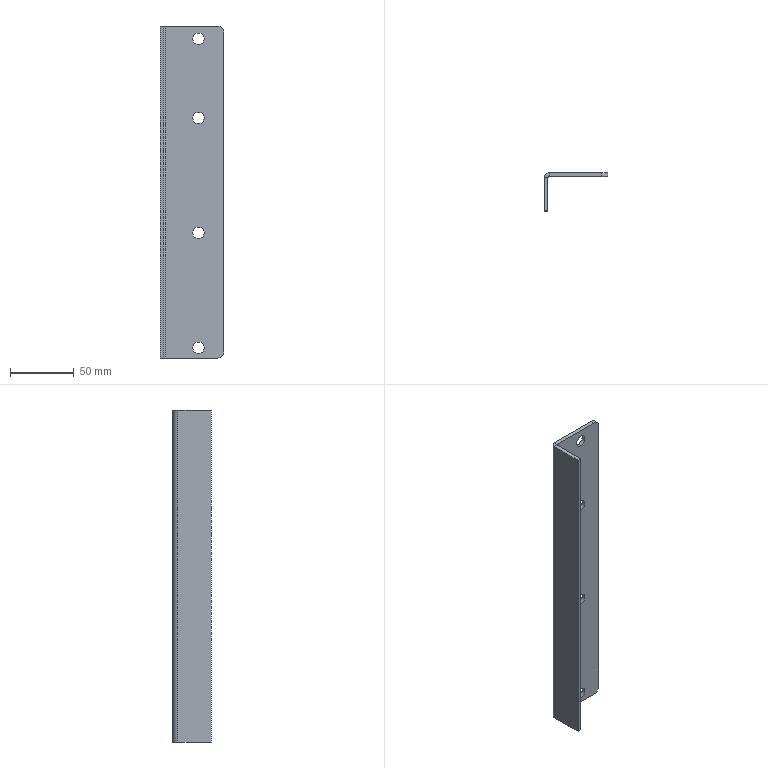Part | SolidWorks | features FlatPattern 1, ICE 1, SMBaseFlange 1, SheetMetal 1 | 1 solid | 24 faces | box 50 x 30 x 260 mm | volume 58427 mm3 | cylinder 12 | plane 12 | commonest cylinder face diameters 9 x8 10 x2 2 x1 8 x1
STEP:
#1=CARTESIAN_POINT('',(30.,27.,3.5));
#2=VERTEX_POINT('',#1);
#3=CARTESIAN_POINT('',(30.,27.,12.5));
#4=VERTEX_POINT('',#3);
#5=CARTESIAN_POINT('',(30.,27.,8.));
#6=DIRECTION('',(0.,1.,0.));
#7=DIRECTION('',(0.,0.,1.));
#8=AXIS2_PLACEMENT_3D('',#5,#6,#7);
#9=CIRCLE('',#8,4.5);
#10=EDGE_CURVE('',#2,#4,#9,.T.);
#11=ORIENTED_EDGE('',*,*,#10,.F.);
#12=CARTESIAN_POINT('',(30.,30.,3.5));
#13=VERTEX_POINT('',#12);
#14=CARTESIAN_POINT('',(30.,30.,3.5));
#15=DIRECTION('',(0.,1.,0.));
#16=VECTOR('',#15,1000.);
#17=LINE('',#14,#16);
#18=EDGE_CURVE('',#2,#13,#17,.T.);
#19=ORIENTED_EDGE('',*,*,#18,.T.);
#20=CARTESIAN_POINT('',(30.,30.,12.5));
#21=VERTEX_POINT('',#20);
#22=CARTESIAN_POINT('',(30.,30.,8.));
#23=DIRECTION('',(0.,1.,0.));
#24=DIRECTION('',(0.,0.,1.));
#25=AXIS2_PLACEMENT_3D('',#22,#23,#24);
#26=CIRCLE('',#25,4.5);
#27=EDGE_CURVE('',#13,#21,#26,.T.);
#28=ORIENTED_EDGE('',*,*,#27,.T.);
#29=CARTESIAN_POINT('',(30.,30.,12.5));
#30=DIRECTION('',(0.,1.,0.));
#31=VECTOR('',#30,1000.);
#32=LINE('',#29,#31);
#33=EDGE_CURVE('',#4,#21,#32,.T.);
#34=ORIENTED_EDGE('',*,*,#33,.F.);
#35=EDGE_LOOP('',(#11,#19,#28,#34));
#36=FACE_OUTER_BOUND('',#35,.T.);
#37=CARTESIAN_POINT('',(30.,30.,8.));
#38=DIRECTION('',(0.,1.,0.));
#39=DIRECTION('',(0.,0.,1.));
#40=AXIS2_PLACEMENT_3D('',#37,#38,#39);
#41=CYLINDRICAL_SURFACE('',#40,4.5);
#42=ADVANCED_FACE('',(#36),#41,.F.);
#43=CARTESIAN_POINT('',(30.,27.,93.5));
#44=VERTEX_POINT('',#43);
#45=CARTESIAN_POINT('',(30.,27.,102.5));
#46=VERTEX_POINT('',#45);
#47=CARTESIAN_POINT('',(30.,27.,98.));
#48=DIRECTION('',(0.,1.,0.));
#49=DIRECTION('',(0.,0.,1.));
#50=AXIS2_PLACEMENT_3D('',#47,#48,#49);
#51=CIRCLE('',#50,4.5);
#52=EDGE_CURVE('',#44,#46,#51,.T.);
#53=ORIENTED_EDGE('',*,*,#52,.F.);
#54=CARTESIAN_POINT('',(30.,30.,93.5));
#55=VERTEX_POINT('',#54);
#56=CARTESIAN_POINT('',(30.,30.,93.5));
#57=DIRECTION('',(0.,1.,0.));
#58=VECTOR('',#57,1000.);
#59=LINE('',#56,#58);
#60=EDGE_CURVE('',#44,#55,#59,.T.);
#61=ORIENTED_EDGE('',*,*,#60,.T.);
#62=CARTESIAN_POINT('',(30.,30.,102.5));
#63=VERTEX_POINT('',#62);
#64=CARTESIAN_POINT('',(30.,30.,98.));
#65=DIRECTION('',(0.,1.,0.));
#66=DIRECTION('',(0.,0.,1.));
#67=AXIS2_PLACEMENT_3D('',#64,#65,#66);
#68=CIRCLE('',#67,4.5);
#69=EDGE_CURVE('',#55,#63,#68,.T.);
#70=ORIENTED_EDGE('',*,*,#69,.T.);
#71=CARTESIAN_POINT('',(30.,30.,102.5));
#72=DIRECTION('',(0.,1.,0.));
#73=VECTOR('',#72,1000.);
#74=LINE('',#71,#73);
#75=EDGE_CURVE('',#46,#63,#74,.T.);
#76=ORIENTED_EDGE('',*,*,#75,.F.);
#77=EDGE_LOOP('',(#53,#61,#70,#76));
#78=FACE_OUTER_BOUND('',#77,.T.);
#79=CARTESIAN_POINT('',(30.,30.,98.));
#80=DIRECTION('',(0.,1.,0.));
#81=DIRECTION('',(0.,0.,1.));
#82=AXIS2_PLACEMENT_3D('',#79,#80,#81);
#83=CYLINDRICAL_SURFACE('',#82,4.5);
#84=ADVANCED_FACE('',(#78),#83,.F.);
#85=CARTESIAN_POINT('',(30.,27.,183.5));
#86=VERTEX_POINT('',#85);
#87=CARTESIAN_POINT('',(30.,27.,192.5));
#88=VERTEX_POINT('',#87);
#89=CARTESIAN_POINT('',(30.,27.,188.));
#90=DIRECTION('',(0.,1.,0.));
#91=DIRECTION('',(0.,0.,1.));
#92=AXIS2_PLACEMENT_3D('',#89,#90,#91);
#93=CIRCLE('',#92,4.5);
#94=EDGE_CURVE('',#86,#88,#93,.T.);
#95=ORIENTED_EDGE('',*,*,#94,.F.);
#96=CARTESIAN_POINT('',(30.,30.,183.5));
#97=VERTEX_POINT('',#96);
#98=CARTESIAN_POINT('',(30.,30.,183.5));
#99=DIRECTION('',(0.,1.,0.));
#100=VECTOR('',#99,1000.);
#101=LINE('',#98,#100);
#102=EDGE_CURVE('',#86,#97,#101,.T.);
#103=ORIENTED_EDGE('',*,*,#102,.T.);
#104=CARTESIAN_POINT('',(30.,30.,192.5));
#105=VERTEX_POINT('',#104);
#106=CARTESIAN_POINT('',(30.,30.,188.));
#107=DIRECTION('',(0.,1.,0.));
#108=DIRECTION('',(0.,0.,1.));
#109=AXIS2_PLACEMENT_3D('',#106,#107,#108);
#110=CIRCLE('',#109,4.5);
#111=EDGE_CURVE('',#97,#105,#110,.T.);
#112=ORIENTED_EDGE('',*,*,#111,.T.);
#113=CARTESIAN_POINT('',(30.,30.,192.5));
#114=DIRECTION('',(0.,1.,0.));
#115=VECTOR('',#114,1000.);
#116=LINE('',#113,#115);
#117=EDGE_CURVE('',#88,#105,#116,.T.);
#118=ORIENTED_EDGE('',*,*,#117,.F.);
#119=EDGE_LOOP('',(#95,#103,#112,#118));
#120=FACE_OUTER_BOUND('',#119,.T.);
#121=CARTESIAN_POINT('',(30.,30.,188.));
#122=DIRECTION('',(0.,1.,0.));
#123=DIRECTION('',(0.,0.,1.));
#124=AXIS2_PLACEMENT_3D('',#121,#122,#123);
#125=CYLINDRICAL_SURFACE('',#124,4.5);
#126=ADVANCED_FACE('',(#120),#125,.F.);
#127=CARTESIAN_POINT('',(30.,27.,245.5));
#128=VERTEX_POINT('',#127);
#129=CARTESIAN_POINT('',(30.,27.,254.5));
#130=VERTEX_POINT('',#129);
#131=CARTESIAN_POINT('',(30.,27.,250.));
#132=DIRECTION('',(0.,1.,0.));
#133=DIRECTION('',(0.,0.,1.));
#134=AXIS2_PLACEMENT_3D('',#131,#132,#133);
#135=CIRCLE('',#134,4.5);
#136=EDGE_CURVE('',#128,#130,#135,.T.);
#137=ORIENTED_EDGE('',*,*,#136,.F.);
#138=CARTESIAN_POINT('',(30.,30.,245.5));
#139=VERTEX_POINT('',#138);
#140=CARTESIAN_POINT('',(30.,30.,245.5));
#141=DIRECTION('',(0.,1.,0.));
#142=VECTOR('',#141,1000.);
#143=LINE('',#140,#142);
#144=EDGE_CURVE('',#128,#139,#143,.T.);
#145=ORIENTED_EDGE('',*,*,#144,.T.);
#146=CARTESIAN_POINT('',(30.,30.,254.5));
#147=VERTEX_POINT('',#146);
#148=CARTESIAN_POINT('',(30.,30.,250.));
#149=DIRECTION('',(0.,1.,0.));
#150=DIRECTION('',(0.,0.,1.));
#151=AXIS2_PLACEMENT_3D('',#148,#149,#150);
#152=CIRCLE('',#151,4.5);
#153=EDGE_CURVE('',#139,#147,#152,.T.);
#154=ORIENTED_EDGE('',*,*,#153,.T.);
#155=CARTESIAN_POINT('',(30.,30.,254.5));
#156=DIRECTION('',(0.,1.,0.));
#157=VECTOR('',#156,1000.);
#158=LINE('',#155,#157);
#159=EDGE_CURVE('',#130,#147,#158,.T.);
#160=ORIENTED_EDGE('',*,*,#159,.F.);
#161=EDGE_LOOP('',(#137,#145,#154,#160));
#162=FACE_OUTER_BOUND('',#161,.T.);
#163=CARTESIAN_POINT('',(30.,30.,250.));
#164=DIRECTION('',(0.,1.,0.));
#165=DIRECTION('',(0.,0.,1.));
#166=AXIS2_PLACEMENT_3D('',#163,#164,#165);
#167=CYLINDRICAL_SURFACE('',#166,4.5);
#168=ADVANCED_FACE('',(#162),#167,.F.);
#169=CARTESIAN_POINT('',(30.,27.,8.));
#170=DIRECTION('',(0.,1.,0.));
#171=DIRECTION('',(0.,0.,1.));
#172=AXIS2_PLACEMENT_3D('',#169,#170,#171);
#173=CIRCLE('',#172,4.5);
#174=EDGE_CURVE('',#4,#2,#173,.T.);
#175=ORIENTED_EDGE('',*,*,#174,.T.);
#176=ORIENTED_EDGE('',*,*,#10,.T.);
#177=EDGE_LOOP('',(#175,#176));
#178=FACE_BOUND('',#177,.T.);
#179=CARTESIAN_POINT('',(30.,27.,98.));
#180=DIRECTION('',(0.,1.,0.));
#181=DIRECTION('',(0.,0.,1.));
#182=AXIS2_PLACEMENT_3D('',#179,#180,#181);
#183=CIRCLE('',#182,4.5);
#184=EDGE_CURVE('',#46,#44,#183,.T.);
#185=ORIENTED_EDGE('',*,*,#184,.T.);
#186=ORIENTED_EDGE('',*,*,#52,.T.);
#187=EDGE_LOOP('',(#185,#186));
#188=FACE_BOUND('',#187,.T.);
#189=CARTESIAN_POINT('',(30.,27.,188.));
#190=DIRECTION('',(0.,1.,0.));
#191=DIRECTION('',(0.,0.,1.));
#192=AXIS2_PLACEMENT_3D('',#189,#190,#191);
#193=CIRCLE('',#192,4.5);
#194=EDGE_CURVE('',#88,#86,#193,.T.);
#195=ORIENTED_EDGE('',*,*,#194,.T.);
#196=ORIENTED_EDGE('',*,*,#94,.T.);
#197=EDGE_LOOP('',(#195,#196));
#198=FACE_BOUND('',#197,.T.);
#199=CARTESIAN_POINT('',(30.,27.,250.));
#200=DIRECTION('',(0.,1.,0.));
#201=DIRECTION('',(0.,0.,1.));
#202=AXIS2_PLACEMENT_3D('',#199,#200,#201);
#203=CIRCLE('',#202,4.5);
#204=EDGE_CURVE('',#130,#128,#203,.T.);
#205=ORIENTED_EDGE('',*,*,#204,.T.);
#206=ORIENTED_EDGE('',*,*,#136,.T.);
#207=EDGE_LOOP('',(#205,#206));
#208=FACE_BOUND('',#207,.T.);
#209=CARTESIAN_POINT('',(45.,27.,0.));
#210=VERTEX_POINT('',#209);
#211=CARTESIAN_POINT('',(50.,27.,5.));
#212=VERTEX_POINT('',#211);
#213=CARTESIAN_POINT('',(45.,27.,5.));
#214=DIRECTION('',(0.,-1.,0.));
#215=DIRECTION('',(0.,0.,1.));
#216=AXIS2_PLACEMENT_3D('',#213,#214,#215);
#217=CIRCLE('',#216,5.);
#218=EDGE_CURVE('',#210,#212,#217,.T.);
#219=ORIENTED_EDGE('',*,*,#218,.T.);
#220=CARTESIAN_POINT('',(50.,27.,255.));
#221=VERTEX_POINT('',#220);
#222=CARTESIAN_POINT('',(50.,27.,260.));
#223=DIRECTION('',(0.,0.,-1.));
#224=VECTOR('',#223,1000.);
#225=LINE('',#222,#224);
#226=EDGE_CURVE('',#221,#212,#225,.T.);
#227=ORIENTED_EDGE('',*,*,#226,.F.);
#228=CARTESIAN_POINT('',(45.,27.,260.));
#229=VERTEX_POINT('',#228);
#230=CARTESIAN_POINT('',(45.,27.,255.));
#231=DIRECTION('',(0.,-1.,0.));
#232=DIRECTION('',(0.,0.,1.));
#233=AXIS2_PLACEMENT_3D('',#230,#231,#232);
#234=CIRCLE('',#233,5.);
#235=EDGE_CURVE('',#221,#229,#234,.T.);
#236=ORIENTED_EDGE('',*,*,#235,.T.);
#237=CARTESIAN_POINT('',(4.,27.,260.));
#238=VERTEX_POINT('',#237);
#239=CARTESIAN_POINT('',(0.,27.,260.));
#240=DIRECTION('',(1.,0.,0.));
#241=VECTOR('',#240,1000.);
#242=LINE('',#239,#241);
#243=EDGE_CURVE('',#238,#229,#242,.T.);
#244=ORIENTED_EDGE('',*,*,#243,.F.);
#245=CARTESIAN_POINT('',(4.,27.,0.));
#246=VERTEX_POINT('',#245);
#247=CARTESIAN_POINT('',(4.,27.,260.));
#248=DIRECTION('',(0.,0.,-1.));
#249=VECTOR('',#248,1000.);
#250=LINE('',#247,#249);
#251=EDGE_CURVE('',#238,#246,#250,.T.);
#252=ORIENTED_EDGE('',*,*,#251,.T.);
#253=CARTESIAN_POINT('',(0.,27.,0.));
#254=DIRECTION('',(1.,0.,0.));
#255=VECTOR('',#254,1000.);
#256=LINE('',#253,#255);
#257=EDGE_CURVE('',#246,#210,#256,.T.);
#258=ORIENTED_EDGE('',*,*,#257,.T.);
#259=EDGE_LOOP('',(#219,#227,#236,#244,#252,#258));
#260=FACE_OUTER_BOUND('',#259,.T.);
#261=CARTESIAN_POINT('',(0.,27.,260.));
#262=DIRECTION('',(0.,1.,0.));
#263=DIRECTION('',(0.,0.,1.));
#264=AXIS2_PLACEMENT_3D('',#261,#262,#263);
#265=PLANE('',#264);
#266=ADVANCED_FACE('',(#178,#188,#198,#208,#260),#265,.F.);
#267=CARTESIAN_POINT('',(30.,30.,8.));
#268=DIRECTION('',(0.,1.,0.));
#269=DIRECTION('',(0.,0.,1.));
#270=AXIS2_PLACEMENT_3D('',#267,#268,#269);
#271=CIRCLE('',#270,4.5);
#272=EDGE_CURVE('',#21,#13,#271,.T.);
#273=ORIENTED_EDGE('',*,*,#272,.F.);
#274=ORIENTED_EDGE('',*,*,#27,.F.);
#275=EDGE_LOOP('',(#273,#274));
#276=FACE_BOUND('',#275,.T.);
#277=CARTESIAN_POINT('',(30.,30.,98.));
#278=DIRECTION('',(0.,1.,0.));
#279=DIRECTION('',(0.,0.,1.));
#280=AXIS2_PLACEMENT_3D('',#277,#278,#279);
#281=CIRCLE('',#280,4.5);
#282=EDGE_CURVE('',#63,#55,#281,.T.);
#283=ORIENTED_EDGE('',*,*,#282,.F.);
#284=ORIENTED_EDGE('',*,*,#69,.F.);
#285=EDGE_LOOP('',(#283,#284));
#286=FACE_BOUND('',#285,.T.);
#287=CARTESIAN_POINT('',(30.,30.,188.));
#288=DIRECTION('',(0.,1.,0.));
#289=DIRECTION('',(0.,0.,1.));
#290=AXIS2_PLACEMENT_3D('',#287,#288,#289);
#291=CIRCLE('',#290,4.5);
#292=EDGE_CURVE('',#105,#97,#291,.T.);
#293=ORIENTED_EDGE('',*,*,#292,.F.);
#294=ORIENTED_EDGE('',*,*,#111,.F.);
#295=EDGE_LOOP('',(#293,#294));
#296=FACE_BOUND('',#295,.T.);
#297=CARTESIAN_POINT('',(30.,30.,250.));
#298=DIRECTION('',(0.,1.,0.));
#299=DIRECTION('',(0.,0.,1.));
#300=AXIS2_PLACEMENT_3D('',#297,#298,#299);
#301=CIRCLE('',#300,4.5);
#302=EDGE_CURVE('',#147,#139,#301,.T.);
#303=ORIENTED_EDGE('',*,*,#302,.F.);
#304=ORIENTED_EDGE('',*,*,#153,.F.);
#305=EDGE_LOOP('',(#303,#304));
#306=FACE_BOUND('',#305,.T.);
#307=CARTESIAN_POINT('',(50.,30.,255.));
#308=VERTEX_POINT('',#307);
#309=CARTESIAN_POINT('',(50.,30.,5.));
#310=VERTEX_POINT('',#309);
#311=CARTESIAN_POINT('',(50.,30.,260.));
#312=DIRECTION('',(0.,0.,-1.));
#313=VECTOR('',#312,1000.);
#314=LINE('',#311,#313);
#315=EDGE_CURVE('',#308,#310,#314,.T.);
#316=ORIENTED_EDGE('',*,*,#315,.T.);
#317=CARTESIAN_POINT('',(45.,30.,0.));
#318=VERTEX_POINT('',#317);
#319=CARTESIAN_POINT('',(45.,30.,5.));
#320=DIRECTION('',(0.,-1.,0.));
#321=DIRECTION('',(0.,0.,1.));
#322=AXIS2_PLACEMENT_3D('',#319,#320,#321);
#323=CIRCLE('',#322,5.);
#324=EDGE_CURVE('',#318,#310,#323,.T.);
#325=ORIENTED_EDGE('',*,*,#324,.F.);
#326=CARTESIAN_POINT('',(4.,30.,0.));
#327=VERTEX_POINT('',#326);
#328=CARTESIAN_POINT('',(0.,30.,0.));
#329=DIRECTION('',(1.,0.,0.));
#330=VECTOR('',#329,1000.);
#331=LINE('',#328,#330);
#332=EDGE_CURVE('',#327,#318,#331,.T.);
#333=ORIENTED_EDGE('',*,*,#332,.F.);
#334=CARTESIAN_POINT('',(4.,30.,260.));
#335=VERTEX_POINT('',#334);
#336=CARTESIAN_POINT('',(4.,30.,260.));
#337=DIRECTION('',(0.,0.,-1.));
#338=VECTOR('',#337,1000.);
#339=LINE('',#336,#338);
#340=EDGE_CURVE('',#335,#327,#339,.T.);
#341=ORIENTED_EDGE('',*,*,#340,.F.);
#342=CARTESIAN_POINT('',(45.,30.,260.));
#343=VERTEX_POINT('',#342);
#344=CARTESIAN_POINT('',(0.,30.,260.));
#345=DIRECTION('',(1.,0.,0.));
#346=VECTOR('',#345,1000.);
#347=LINE('',#344,#346);
#348=EDGE_CURVE('',#335,#343,#347,.T.);
#349=ORIENTED_EDGE('',*,*,#348,.T.);
#350=CARTESIAN_POINT('',(45.,30.,255.));
#351=DIRECTION('',(0.,-1.,0.));
#352=DIRECTION('',(0.,0.,1.));
#353=AXIS2_PLACEMENT_3D('',#350,#351,#352);
#354=CIRCLE('',#353,5.);
#355=EDGE_CURVE('',#308,#343,#354,.T.);
#356=ORIENTED_EDGE('',*,*,#355,.F.);
#357=EDGE_LOOP('',(#316,#325,#333,#341,#349,#356));
#358=FACE_OUTER_BOUND('',#357,.T.);
#359=CARTESIAN_POINT('',(0.,30.,260.));
#360=DIRECTION('',(0.,1.,0.));
#361=DIRECTION('',(0.,0.,1.));
#362=AXIS2_PLACEMENT_3D('',#359,#360,#361);
#363=PLANE('',#362);
#364=ADVANCED_FACE('',(#276,#286,#296,#306,#358),#363,.T.);
#365=ORIENTED_EDGE('',*,*,#226,.T.);
#366=CARTESIAN_POINT('',(50.,30.,5.));
#367=DIRECTION('',(0.,-1.,0.));
#368=VECTOR('',#367,1000.);
#369=LINE('',#366,#368);
#370=EDGE_CURVE('',#310,#212,#369,.T.);
#371=ORIENTED_EDGE('',*,*,#370,.F.);
#372=ORIENTED_EDGE('',*,*,#315,.F.);
#373=CARTESIAN_POINT('',(50.,30.,255.));
#374=DIRECTION('',(0.,-1.,0.));
#375=VECTOR('',#374,1000.);
#376=LINE('',#373,#375);
#377=EDGE_CURVE('',#308,#221,#376,.T.);
#378=ORIENTED_EDGE('',*,*,#377,.T.);
#379=EDGE_LOOP('',(#365,#371,#372,#378));
#380=FACE_OUTER_BOUND('',#379,.T.);
#381=CARTESIAN_POINT('',(50.,30.,260.));
#382=DIRECTION('',(1.,0.,0.));
#383=DIRECTION('',(0.,0.,-1.));
#384=AXIS2_PLACEMENT_3D('',#381,#382,#383);
#385=PLANE('',#384);
#386=ADVANCED_FACE('',(#380),#385,.T.);
#387=CARTESIAN_POINT('',(45.,30.,0.));
#388=DIRECTION('',(0.,-1.,0.));
#389=VECTOR('',#388,1000.);
#390=LINE('',#387,#389);
#391=EDGE_CURVE('',#318,#210,#390,.T.);
#392=ORIENTED_EDGE('',*,*,#391,.T.);
#393=ORIENTED_EDGE('',*,*,#257,.F.);
#394=CARTESIAN_POINT('',(4.,27.,0.));
#395=DIRECTION('',(0.,1.,0.));
#396=VECTOR('',#395,1000.);
#397=LINE('',#394,#396);
#398=EDGE_CURVE('',#246,#327,#397,.T.);
#399=ORIENTED_EDGE('',*,*,#398,.T.);
#400=ORIENTED_EDGE('',*,*,#332,.T.);
#401=EDGE_LOOP('',(#392,#393,#399,#400));
#402=FACE_OUTER_BOUND('',#401,.T.);
#403=CARTESIAN_POINT('',(4.,26.,0.));
#404=DIRECTION('',(0.,0.,1.));
#405=DIRECTION('',(1.,0.,0.));
#406=AXIS2_PLACEMENT_3D('',#403,#404,#405);
#407=PLANE('',#406);
#408=ADVANCED_FACE('',(#402),#407,.F.);
#409=ORIENTED_EDGE('',*,*,#243,.T.);
#410=CARTESIAN_POINT('',(45.,30.,260.));
#411=DIRECTION('',(0.,-1.,0.));
#412=VECTOR('',#411,1000.);
#413=LINE('',#410,#412);
#414=EDGE_CURVE('',#343,#229,#413,.T.);
#415=ORIENTED_EDGE('',*,*,#414,.F.);
#416=ORIENTED_EDGE('',*,*,#348,.F.);
#417=CARTESIAN_POINT('',(4.,30.,260.));
#418=DIRECTION('',(0.,-1.,0.));
#419=VECTOR('',#418,1000.);
#420=LINE('',#417,#419);
#421=EDGE_CURVE('',#335,#238,#420,.T.);
#422=ORIENTED_EDGE('',*,*,#421,.T.);
#423=EDGE_LOOP('',(#409,#415,#416,#422));
#424=FACE_OUTER_BOUND('',#423,.T.);
#425=CARTESIAN_POINT('',(3.,26.,260.));
#426=DIRECTION('',(0.,0.,1.));
#427=DIRECTION('',(1.,0.,0.));
#428=AXIS2_PLACEMENT_3D('',#425,#426,#427);
#429=PLANE('',#428);
#430=ADVANCED_FACE('',(#424),#429,.T.);
#431=ORIENTED_EDGE('',*,*,#421,.F.);
#432=CARTESIAN_POINT('',(0.,26.,260.));
#433=VERTEX_POINT('',#432);
#434=CARTESIAN_POINT('',(4.,26.,260.));
#435=DIRECTION('',(0.,0.,-1.));
#436=DIRECTION('',(1.,0.,0.));
#437=AXIS2_PLACEMENT_3D('',#434,#435,#436);
#438=CIRCLE('',#437,4.);
#439=EDGE_CURVE('',#433,#335,#438,.T.);
#440=ORIENTED_EDGE('',*,*,#439,.F.);
#441=CARTESIAN_POINT('',(3.,26.,260.));
#442=VERTEX_POINT('',#441);
#443=CARTESIAN_POINT('',(3.,26.,260.));
#444=DIRECTION('',(-1.,0.,0.));
#445=VECTOR('',#444,1000.);
#446=LINE('',#443,#445);
#447=EDGE_CURVE('',#442,#433,#446,.T.);
#448=ORIENTED_EDGE('',*,*,#447,.F.);
#449=CARTESIAN_POINT('',(4.,26.,260.));
#450=DIRECTION('',(0.,0.,-1.));
#451=DIRECTION('',(1.,0.,0.));
#452=AXIS2_PLACEMENT_3D('',#449,#450,#451);
#453=CIRCLE('',#452,1.);
#454=EDGE_CURVE('',#442,#238,#453,.T.);
#455=ORIENTED_EDGE('',*,*,#454,.T.);
#456=EDGE_LOOP('',(#431,#440,#448,#455));
#457=FACE_OUTER_BOUND('',#456,.T.);
#458=CARTESIAN_POINT('',(4.,30.,260.));
#459=DIRECTION('',(0.,0.,1.));
#460=DIRECTION('',(1.,0.,0.));
#461=AXIS2_PLACEMENT_3D('',#458,#459,#460);
#462=PLANE('',#461);
#463=ADVANCED_FACE('',(#457),#462,.T.);
#464=CARTESIAN_POINT('',(0.,26.,0.));
#465=VERTEX_POINT('',#464);
#466=CARTESIAN_POINT('',(3.,26.,0.));
#467=VERTEX_POINT('',#466);
#468=CARTESIAN_POINT('',(0.,26.,0.));
#469=DIRECTION('',(1.,0.,0.));
#470=VECTOR('',#469,1000.);
#471=LINE('',#468,#470);
#472=EDGE_CURVE('',#465,#467,#471,.T.);
#473=ORIENTED_EDGE('',*,*,#472,.F.);
#474=CARTESIAN_POINT('',(4.,26.,0.));
#475=DIRECTION('',(0.,0.,-1.));
#476=DIRECTION('',(1.,0.,0.));
#477=AXIS2_PLACEMENT_3D('',#474,#475,#476);
#478=CIRCLE('',#477,4.);
#479=EDGE_CURVE('',#465,#327,#478,.T.);
#480=ORIENTED_EDGE('',*,*,#479,.T.);
#481=ORIENTED_EDGE('',*,*,#398,.F.);
#482=CARTESIAN_POINT('',(4.,26.,0.));
#483=DIRECTION('',(0.,0.,-1.));
#484=DIRECTION('',(1.,0.,0.));
#485=AXIS2_PLACEMENT_3D('',#482,#483,#484);
#486=CIRCLE('',#485,1.);
#487=EDGE_CURVE('',#467,#246,#486,.T.);
#488=ORIENTED_EDGE('',*,*,#487,.F.);
#489=EDGE_LOOP('',(#473,#480,#481,#488));
#490=FACE_OUTER_BOUND('',#489,.T.);
#491=CARTESIAN_POINT('',(0.,26.,0.));
#492=DIRECTION('',(0.,0.,-1.));
#493=DIRECTION('',(-1.,0.,0.));
#494=AXIS2_PLACEMENT_3D('',#491,#492,#493);
#495=PLANE('',#494);
#496=ADVANCED_FACE('',(#490),#495,.T.);
#497=CARTESIAN_POINT('',(0.,0.,0.));
#498=VERTEX_POINT('',#497);
#499=CARTESIAN_POINT('',(0.,0.,0.));
#500=DIRECTION('',(0.,1.,0.));
#501=VECTOR('',#500,1000.);
#502=LINE('',#499,#501);
#503=EDGE_CURVE('',#498,#465,#502,.T.);
#504=ORIENTED_EDGE('',*,*,#503,.T.);
#505=ORIENTED_EDGE('',*,*,#472,.T.);
#506=CARTESIAN_POINT('',(3.,0.,0.));
#507=VERTEX_POINT('',#506);
#508=CARTESIAN_POINT('',(3.,0.,0.));
#509=DIRECTION('',(0.,1.,0.));
#510=VECTOR('',#509,1000.);
#511=LINE('',#508,#510);
#512=EDGE_CURVE('',#507,#467,#511,.T.);
#513=ORIENTED_EDGE('',*,*,#512,.F.);
#514=CARTESIAN_POINT('',(3.,0.,0.));
#515=DIRECTION('',(-1.,0.,0.));
#516=VECTOR('',#515,1000.);
#517=LINE('',#514,#516);
#518=EDGE_CURVE('',#507,#498,#517,.T.);
#519=ORIENTED_EDGE('',*,*,#518,.T.);
#520=EDGE_LOOP('',(#504,#505,#513,#519));
#521=FACE_OUTER_BOUND('',#520,.T.);
#522=CARTESIAN_POINT('',(4.,27.,0.));
#523=DIRECTION('',(0.,0.,-1.));
#524=DIRECTION('',(-1.,0.,0.));
#525=AXIS2_PLACEMENT_3D('',#522,#523,#524);
#526=PLANE('',#525);
#527=ADVANCED_FACE('',(#521),#526,.T.);
#528=ORIENTED_EDGE('',*,*,#479,.F.);
#529=CARTESIAN_POINT('',(0.,26.,260.));
#530=DIRECTION('',(0.,0.,-1.));
#531=VECTOR('',#530,1000.);
#532=LINE('',#529,#531);
#533=EDGE_CURVE('',#433,#465,#532,.T.);
#534=ORIENTED_EDGE('',*,*,#533,.F.);
#535=ORIENTED_EDGE('',*,*,#439,.T.);
#536=ORIENTED_EDGE('',*,*,#340,.T.);
#537=EDGE_LOOP('',(#528,#534,#535,#536));
#538=FACE_OUTER_BOUND('',#537,.T.);
#539=CARTESIAN_POINT('',(4.,26.,260.));
#540=DIRECTION('',(0.,0.,-1.));
#541=DIRECTION('',(-1.,0.,0.));
#542=AXIS2_PLACEMENT_3D('',#539,#540,#541);
#543=CYLINDRICAL_SURFACE('',#542,4.);
#544=ADVANCED_FACE('',(#538),#543,.T.);
#545=ORIENTED_EDGE('',*,*,#503,.F.);
#546=CARTESIAN_POINT('',(0.,0.,260.));
#547=VERTEX_POINT('',#546);
#548=CARTESIAN_POINT('',(0.,0.,260.));
#549=DIRECTION('',(0.,0.,-1.));
#550=VECTOR('',#549,1000.);
#551=LINE('',#548,#550);
#552=EDGE_CURVE('',#547,#498,#551,.T.);
#553=ORIENTED_EDGE('',*,*,#552,.F.);
#554=CARTESIAN_POINT('',(0.,0.,260.));
#555=DIRECTION('',(0.,1.,0.));
#556=VECTOR('',#555,1000.);
#557=LINE('',#554,#556);
#558=EDGE_CURVE('',#547,#433,#557,.T.);
#559=ORIENTED_EDGE('',*,*,#558,.T.);
#560=ORIENTED_EDGE('',*,*,#533,.T.);
#561=EDGE_LOOP('',(#545,#553,#559,#560));
#562=FACE_OUTER_BOUND('',#561,.T.);
#563=CARTESIAN_POINT('',(0.,0.,260.));
#564=DIRECTION('',(-1.,0.,0.));
#565=DIRECTION('',(0.,0.,1.));
#566=AXIS2_PLACEMENT_3D('',#563,#564,#565);
#567=PLANE('',#566);
#568=ADVANCED_FACE('',(#562),#567,.T.);
#569=ORIENTED_EDGE('',*,*,#518,.F.);
#570=CARTESIAN_POINT('',(3.,0.,260.));
#571=VERTEX_POINT('',#570);
#572=CARTESIAN_POINT('',(3.,0.,260.));
#573=DIRECTION('',(0.,0.,-1.));
#574=VECTOR('',#573,1000.);
#575=LINE('',#572,#574);
#576=EDGE_CURVE('',#571,#507,#575,.T.);
#577=ORIENTED_EDGE('',*,*,#576,.F.);
#578=CARTESIAN_POINT('',(3.,0.,260.));
#579=DIRECTION('',(-1.,0.,0.));
#580=VECTOR('',#579,1000.);
#581=LINE('',#578,#580);
#582=EDGE_CURVE('',#571,#547,#581,.T.);
#583=ORIENTED_EDGE('',*,*,#582,.T.);
#584=ORIENTED_EDGE('',*,*,#552,.T.);
#585=EDGE_LOOP('',(#569,#577,#583,#584));
#586=FACE_OUTER_BOUND('',#585,.T.);
#587=CARTESIAN_POINT('',(3.,0.,260.));
#588=DIRECTION('',(0.,-1.,0.));
#589=DIRECTION('',(0.,0.,-1.));
#590=AXIS2_PLACEMENT_3D('',#587,#588,#589);
#591=PLANE('',#590);
#592=ADVANCED_FACE('',(#586),#591,.T.);
#593=ORIENTED_EDGE('',*,*,#512,.T.);
#594=CARTESIAN_POINT('',(3.,26.,260.));
#595=DIRECTION('',(0.,0.,-1.));
#596=VECTOR('',#595,1000.);
#597=LINE('',#594,#596);
#598=EDGE_CURVE('',#442,#467,#597,.T.);
#599=ORIENTED_EDGE('',*,*,#598,.F.);
#600=CARTESIAN_POINT('',(3.,0.,260.));
#601=DIRECTION('',(0.,1.,0.));
#602=VECTOR('',#601,1000.);
#603=LINE('',#600,#602);
#604=EDGE_CURVE('',#571,#442,#603,.T.);
#605=ORIENTED_EDGE('',*,*,#604,.F.);
#606=ORIENTED_EDGE('',*,*,#576,.T.);
#607=EDGE_LOOP('',(#593,#599,#605,#606));
#608=FACE_OUTER_BOUND('',#607,.T.);
#609=CARTESIAN_POINT('',(3.,0.,260.));
#610=DIRECTION('',(-1.,0.,0.));
#611=DIRECTION('',(0.,0.,1.));
#612=AXIS2_PLACEMENT_3D('',#609,#610,#611);
#613=PLANE('',#612);
#614=ADVANCED_FACE('',(#608),#613,.F.);
#615=ORIENTED_EDGE('',*,*,#487,.T.);
#616=ORIENTED_EDGE('',*,*,#251,.F.);
#617=ORIENTED_EDGE('',*,*,#454,.F.);
#618=ORIENTED_EDGE('',*,*,#598,.T.);
#619=EDGE_LOOP('',(#615,#616,#617,#618));
#620=FACE_OUTER_BOUND('',#619,.T.);
#621=CARTESIAN_POINT('',(4.,26.,260.));
#622=DIRECTION('',(0.,0.,-1.));
#623=DIRECTION('',(-1.,0.,0.));
#624=AXIS2_PLACEMENT_3D('',#621,#622,#623);
#625=CYLINDRICAL_SURFACE('',#624,1.);
#626=ADVANCED_FACE('',(#620),#625,.F.);
#627=ORIENTED_EDGE('',*,*,#604,.T.);
#628=ORIENTED_EDGE('',*,*,#447,.T.);
#629=ORIENTED_EDGE('',*,*,#558,.F.);
#630=ORIENTED_EDGE('',*,*,#582,.F.);
#631=EDGE_LOOP('',(#627,#628,#629,#630));
#632=FACE_OUTER_BOUND('',#631,.T.);
#633=CARTESIAN_POINT('',(4.,26.,260.));
#634=DIRECTION('',(0.,0.,1.));
#635=DIRECTION('',(1.,0.,0.));
#636=AXIS2_PLACEMENT_3D('',#633,#634,#635);
#637=PLANE('',#636);
#638=ADVANCED_FACE('',(#632),#637,.T.);
#639=ORIENTED_EDGE('',*,*,#144,.F.);
#640=ORIENTED_EDGE('',*,*,#204,.F.);
#641=ORIENTED_EDGE('',*,*,#159,.T.);
#642=ORIENTED_EDGE('',*,*,#302,.T.);
#643=EDGE_LOOP('',(#639,#640,#641,#642));
#644=FACE_OUTER_BOUND('',#643,.T.);
#645=CARTESIAN_POINT('',(30.,30.,250.));
#646=DIRECTION('',(0.,1.,0.));
#647=DIRECTION('',(0.,0.,1.));
#648=AXIS2_PLACEMENT_3D('',#645,#646,#647);
#649=CYLINDRICAL_SURFACE('',#648,4.5);
#650=ADVANCED_FACE('',(#644),#649,.F.);
#651=ORIENTED_EDGE('',*,*,#102,.F.);
#652=ORIENTED_EDGE('',*,*,#194,.F.);
#653=ORIENTED_EDGE('',*,*,#117,.T.);
#654=ORIENTED_EDGE('',*,*,#292,.T.);
#655=EDGE_LOOP('',(#651,#652,#653,#654));
#656=FACE_OUTER_BOUND('',#655,.T.);
#657=CARTESIAN_POINT('',(30.,30.,188.));
#658=DIRECTION('',(0.,1.,0.));
#659=DIRECTION('',(0.,0.,1.));
#660=AXIS2_PLACEMENT_3D('',#657,#658,#659);
#661=CYLINDRICAL_SURFACE('',#660,4.5);
#662=ADVANCED_FACE('',(#656),#661,.F.);
#663=ORIENTED_EDGE('',*,*,#60,.F.);
#664=ORIENTED_EDGE('',*,*,#184,.F.);
#665=ORIENTED_EDGE('',*,*,#75,.T.);
#666=ORIENTED_EDGE('',*,*,#282,.T.);
#667=EDGE_LOOP('',(#663,#664,#665,#666));
#668=FACE_OUTER_BOUND('',#667,.T.);
#669=CARTESIAN_POINT('',(30.,30.,98.));
#670=DIRECTION('',(0.,1.,0.));
#671=DIRECTION('',(0.,0.,1.));
#672=AXIS2_PLACEMENT_3D('',#669,#670,#671);
#673=CYLINDRICAL_SURFACE('',#672,4.5);
#674=ADVANCED_FACE('',(#668),#673,.F.);
#675=ORIENTED_EDGE('',*,*,#18,.F.);
#676=ORIENTED_EDGE('',*,*,#174,.F.);
#677=ORIENTED_EDGE('',*,*,#33,.T.);
#678=ORIENTED_EDGE('',*,*,#272,.T.);
#679=EDGE_LOOP('',(#675,#676,#677,#678));
#680=FACE_OUTER_BOUND('',#679,.T.);
#681=CARTESIAN_POINT('',(30.,30.,8.));
#682=DIRECTION('',(0.,1.,0.));
#683=DIRECTION('',(0.,0.,1.));
#684=AXIS2_PLACEMENT_3D('',#681,#682,#683);
#685=CYLINDRICAL_SURFACE('',#684,4.5);
#686=ADVANCED_FACE('',(#680),#685,.F.);
#687=ORIENTED_EDGE('',*,*,#355,.T.);
#688=ORIENTED_EDGE('',*,*,#414,.T.);
#689=ORIENTED_EDGE('',*,*,#235,.F.);
#690=ORIENTED_EDGE('',*,*,#377,.F.);
#691=EDGE_LOOP('',(#687,#688,#689,#690));
#692=FACE_OUTER_BOUND('',#691,.T.);
#693=CARTESIAN_POINT('',(45.,30.,255.));
#694=DIRECTION('',(0.,1.,0.));
#695=DIRECTION('',(0.,0.,1.));
#696=AXIS2_PLACEMENT_3D('',#693,#694,#695);
#697=CYLINDRICAL_SURFACE('',#696,5.);
#698=ADVANCED_FACE('',(#692),#697,.T.);
#699=ORIENTED_EDGE('',*,*,#324,.T.);
#700=ORIENTED_EDGE('',*,*,#370,.T.);
#701=ORIENTED_EDGE('',*,*,#218,.F.);
#702=ORIENTED_EDGE('',*,*,#391,.F.);
#703=EDGE_LOOP('',(#699,#700,#701,#702));
#704=FACE_OUTER_BOUND('',#703,.T.);
#705=CARTESIAN_POINT('',(45.,30.,5.));
#706=DIRECTION('',(0.,1.,0.));
#707=DIRECTION('',(0.,0.,1.));
#708=AXIS2_PLACEMENT_3D('',#705,#706,#707);
#709=CYLINDRICAL_SURFACE('',#708,5.);
#710=ADVANCED_FACE('',(#704),#709,.T.);
#711=CLOSED_SHELL('',(#42,#84,#126,#168,#266,#364,#386,#408,#430,#463,#496,#527,#544,#568,#592,#614,#626,#638,#650,#662,#674,#686,#698,#710));
#712=MANIFOLD_SOLID_BREP('',#711);
#713=CARTESIAN_POINT('',(0.,0.,0.));
#714=DIRECTION('',(0.,0.,1.));
#715=DIRECTION('',(1.,0.,0.));
#716=AXIS2_PLACEMENT_3D('',#713,#714,#715);
#717=(LENGTH_UNIT()NAMED_UNIT(*)SI_UNIT(.MILLI.,.METRE.));
#718=UNCERTAINTY_MEASURE_WITH_UNIT(LENGTH_MEASURE(0.00001),#717,'','');
#719=(NAMED_UNIT(*)PLANE_ANGLE_UNIT()SI_UNIT($,.RADIAN.));
#720=(NAMED_UNIT(*)SI_UNIT($,.STERADIAN.)SOLID_ANGLE_UNIT());
#721=(GEOMETRIC_REPRESENTATION_CONTEXT(3)GLOBAL_UNCERTAINTY_ASSIGNED_CONTEXT((#718))GLOBAL_UNIT_ASSIGNED_CONTEXT((#717,#719,#720))REPRESENTATION_CONTEXT('',''));
#722=ADVANCED_BREP_SHAPE_REPRESENTATION('',(#712,#716),#721);